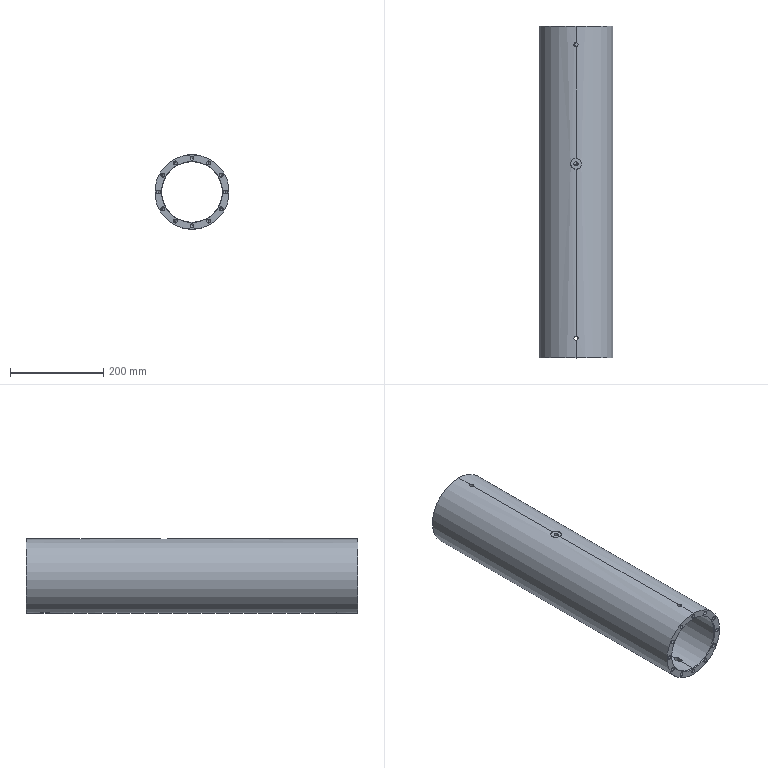Part | SolidWorks | features HoleWzd 5, ICE 5, Chamfer 2, MirrorPattern 2, CirPattern 1, Extrusion 1, LPattern 1 | 1 solid | 234 faces | box 160 x 712.5 x 160 mm | volume 4794263 mm3 | cylinder 150 | cone 56 | plane 28 | commonest cylinder face diameters 8.5 x48 9 x40 15 x38 2.5 x8 10 x6 8.8 x4